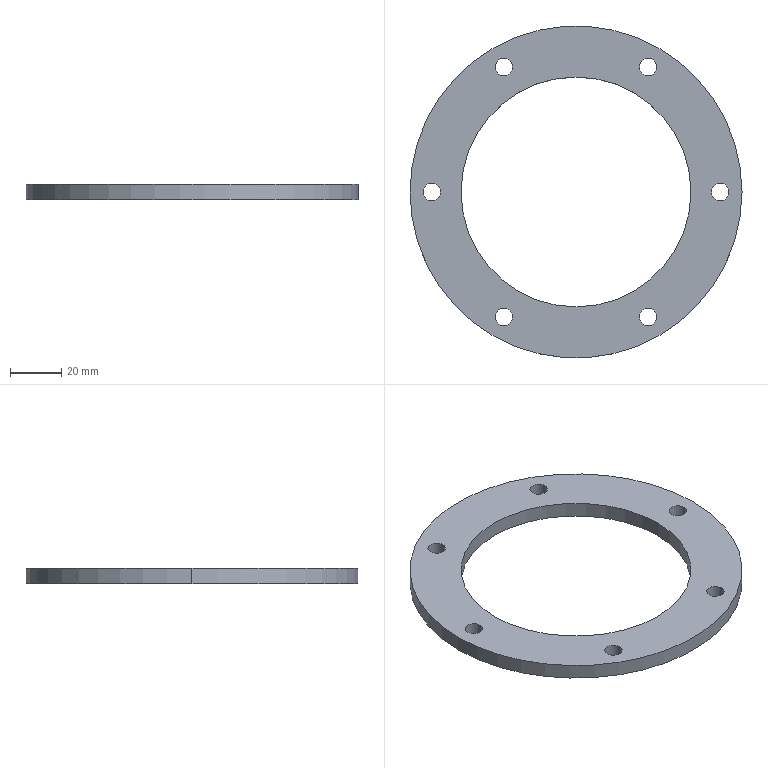Part | SolidWorks | features FlatPattern 1, HoleWzd 1, SMBaseFlange 1, SheetMetal 1 | 1 solid | 18 faces | box 130 x 130 x 6 mm | volume 40162 mm3 | cylinder 16 | plane 2 | commonest cylinder face diameters 6.8 x12 90 x2 130 x2
STEP:
#1=CARTESIAN_POINT('',(-31.65,48.93,-6.));
#2=VERTEX_POINT('',#1);
#3=CARTESIAN_POINT('',(-24.85,48.93,-6.));
#4=VERTEX_POINT('',#3);
#5=CARTESIAN_POINT('',(-28.25,48.93,-6.));
#6=DIRECTION('',(0.,0.,1.));
#7=DIRECTION('',(1.,0.,0.));
#8=AXIS2_PLACEMENT_3D('',#5,#6,#7);
#9=CIRCLE('',#8,3.4);
#10=EDGE_CURVE('',#2,#4,#9,.T.);
#11=ORIENTED_EDGE('',*,*,#10,.F.);
#12=CARTESIAN_POINT('',(-31.65,48.93,0.));
#13=VERTEX_POINT('',#12);
#14=CARTESIAN_POINT('',(-31.65,48.93,0.));
#15=DIRECTION('',(0.,0.,1.));
#16=VECTOR('',#15,1000.);
#17=LINE('',#14,#16);
#18=EDGE_CURVE('',#2,#13,#17,.T.);
#19=ORIENTED_EDGE('',*,*,#18,.T.);
#20=CARTESIAN_POINT('',(-24.85,48.93,0.));
#21=VERTEX_POINT('',#20);
#22=CARTESIAN_POINT('',(-28.25,48.93,0.));
#23=DIRECTION('',(0.,0.,1.));
#24=DIRECTION('',(1.,0.,0.));
#25=AXIS2_PLACEMENT_3D('',#22,#23,#24);
#26=CIRCLE('',#25,3.4);
#27=EDGE_CURVE('',#13,#21,#26,.T.);
#28=ORIENTED_EDGE('',*,*,#27,.T.);
#29=CARTESIAN_POINT('',(-24.85,48.93,0.));
#30=DIRECTION('',(0.,0.,1.));
#31=VECTOR('',#30,1000.);
#32=LINE('',#29,#31);
#33=EDGE_CURVE('',#4,#21,#32,.T.);
#34=ORIENTED_EDGE('',*,*,#33,.F.);
#35=EDGE_LOOP('',(#11,#19,#28,#34));
#36=FACE_OUTER_BOUND('',#35,.T.);
#37=CARTESIAN_POINT('',(-28.25,48.93,0.));
#38=DIRECTION('',(0.,0.,1.));
#39=DIRECTION('',(1.,0.,0.));
#40=AXIS2_PLACEMENT_3D('',#37,#38,#39);
#41=CYLINDRICAL_SURFACE('',#40,3.4);
#42=ADVANCED_FACE('',(#36),#41,.F.);
#43=CARTESIAN_POINT('',(24.85,48.93,-6.));
#44=VERTEX_POINT('',#43);
#45=CARTESIAN_POINT('',(31.65,48.93,-6.));
#46=VERTEX_POINT('',#45);
#47=CARTESIAN_POINT('',(28.25,48.93,-6.));
#48=DIRECTION('',(0.,0.,1.));
#49=DIRECTION('',(1.,0.,0.));
#50=AXIS2_PLACEMENT_3D('',#47,#48,#49);
#51=CIRCLE('',#50,3.4);
#52=EDGE_CURVE('',#44,#46,#51,.T.);
#53=ORIENTED_EDGE('',*,*,#52,.F.);
#54=CARTESIAN_POINT('',(24.85,48.93,0.));
#55=VERTEX_POINT('',#54);
#56=CARTESIAN_POINT('',(24.85,48.93,0.));
#57=DIRECTION('',(0.,0.,1.));
#58=VECTOR('',#57,1000.);
#59=LINE('',#56,#58);
#60=EDGE_CURVE('',#44,#55,#59,.T.);
#61=ORIENTED_EDGE('',*,*,#60,.T.);
#62=CARTESIAN_POINT('',(31.65,48.93,0.));
#63=VERTEX_POINT('',#62);
#64=CARTESIAN_POINT('',(28.25,48.93,0.));
#65=DIRECTION('',(0.,0.,1.));
#66=DIRECTION('',(1.,0.,0.));
#67=AXIS2_PLACEMENT_3D('',#64,#65,#66);
#68=CIRCLE('',#67,3.4);
#69=EDGE_CURVE('',#55,#63,#68,.T.);
#70=ORIENTED_EDGE('',*,*,#69,.T.);
#71=CARTESIAN_POINT('',(31.65,48.93,0.));
#72=DIRECTION('',(0.,0.,1.));
#73=VECTOR('',#72,1000.);
#74=LINE('',#71,#73);
#75=EDGE_CURVE('',#46,#63,#74,.T.);
#76=ORIENTED_EDGE('',*,*,#75,.F.);
#77=EDGE_LOOP('',(#53,#61,#70,#76));
#78=FACE_OUTER_BOUND('',#77,.T.);
#79=CARTESIAN_POINT('',(28.25,48.93,0.));
#80=DIRECTION('',(0.,0.,1.));
#81=DIRECTION('',(1.,0.,0.));
#82=AXIS2_PLACEMENT_3D('',#79,#80,#81);
#83=CYLINDRICAL_SURFACE('',#82,3.4);
#84=ADVANCED_FACE('',(#78),#83,.F.);
#85=CARTESIAN_POINT('',(53.1,0.,-6.));
#86=VERTEX_POINT('',#85);
#87=CARTESIAN_POINT('',(59.9,0.,-6.));
#88=VERTEX_POINT('',#87);
#89=CARTESIAN_POINT('',(56.5,0.,-6.));
#90=DIRECTION('',(0.,0.,1.));
#91=DIRECTION('',(1.,0.,0.));
#92=AXIS2_PLACEMENT_3D('',#89,#90,#91);
#93=CIRCLE('',#92,3.4);
#94=EDGE_CURVE('',#86,#88,#93,.T.);
#95=ORIENTED_EDGE('',*,*,#94,.F.);
#96=CARTESIAN_POINT('',(53.1,0.,0.));
#97=VERTEX_POINT('',#96);
#98=CARTESIAN_POINT('',(53.1,0.,0.));
#99=DIRECTION('',(0.,0.,1.));
#100=VECTOR('',#99,1000.);
#101=LINE('',#98,#100);
#102=EDGE_CURVE('',#86,#97,#101,.T.);
#103=ORIENTED_EDGE('',*,*,#102,.T.);
#104=CARTESIAN_POINT('',(59.9,0.,0.));
#105=VERTEX_POINT('',#104);
#106=CARTESIAN_POINT('',(56.5,0.,0.));
#107=DIRECTION('',(0.,0.,1.));
#108=DIRECTION('',(1.,0.,0.));
#109=AXIS2_PLACEMENT_3D('',#106,#107,#108);
#110=CIRCLE('',#109,3.4);
#111=EDGE_CURVE('',#97,#105,#110,.T.);
#112=ORIENTED_EDGE('',*,*,#111,.T.);
#113=CARTESIAN_POINT('',(59.9,0.,0.));
#114=DIRECTION('',(0.,0.,1.));
#115=VECTOR('',#114,1000.);
#116=LINE('',#113,#115);
#117=EDGE_CURVE('',#88,#105,#116,.T.);
#118=ORIENTED_EDGE('',*,*,#117,.F.);
#119=EDGE_LOOP('',(#95,#103,#112,#118));
#120=FACE_OUTER_BOUND('',#119,.T.);
#121=CARTESIAN_POINT('',(56.5,0.,0.));
#122=DIRECTION('',(0.,0.,1.));
#123=DIRECTION('',(1.,0.,0.));
#124=AXIS2_PLACEMENT_3D('',#121,#122,#123);
#125=CYLINDRICAL_SURFACE('',#124,3.4);
#126=ADVANCED_FACE('',(#120),#125,.F.);
#127=CARTESIAN_POINT('',(-59.9,0.,-6.));
#128=VERTEX_POINT('',#127);
#129=CARTESIAN_POINT('',(-53.1,0.,-6.));
#130=VERTEX_POINT('',#129);
#131=CARTESIAN_POINT('',(-56.5,0.,-6.));
#132=DIRECTION('',(0.,0.,1.));
#133=DIRECTION('',(1.,0.,0.));
#134=AXIS2_PLACEMENT_3D('',#131,#132,#133);
#135=CIRCLE('',#134,3.4);
#136=EDGE_CURVE('',#128,#130,#135,.T.);
#137=ORIENTED_EDGE('',*,*,#136,.F.);
#138=CARTESIAN_POINT('',(-59.9,0.,0.));
#139=VERTEX_POINT('',#138);
#140=CARTESIAN_POINT('',(-59.9,0.,0.));
#141=DIRECTION('',(0.,0.,1.));
#142=VECTOR('',#141,1000.);
#143=LINE('',#140,#142);
#144=EDGE_CURVE('',#128,#139,#143,.T.);
#145=ORIENTED_EDGE('',*,*,#144,.T.);
#146=CARTESIAN_POINT('',(-53.1,0.,0.));
#147=VERTEX_POINT('',#146);
#148=CARTESIAN_POINT('',(-56.5,0.,0.));
#149=DIRECTION('',(0.,0.,1.));
#150=DIRECTION('',(1.,0.,0.));
#151=AXIS2_PLACEMENT_3D('',#148,#149,#150);
#152=CIRCLE('',#151,3.4);
#153=EDGE_CURVE('',#139,#147,#152,.T.);
#154=ORIENTED_EDGE('',*,*,#153,.T.);
#155=CARTESIAN_POINT('',(-53.1,0.,0.));
#156=DIRECTION('',(0.,0.,1.));
#157=VECTOR('',#156,1000.);
#158=LINE('',#155,#157);
#159=EDGE_CURVE('',#130,#147,#158,.T.);
#160=ORIENTED_EDGE('',*,*,#159,.F.);
#161=EDGE_LOOP('',(#137,#145,#154,#160));
#162=FACE_OUTER_BOUND('',#161,.T.);
#163=CARTESIAN_POINT('',(-56.5,0.,0.));
#164=DIRECTION('',(0.,0.,1.));
#165=DIRECTION('',(1.,0.,0.));
#166=AXIS2_PLACEMENT_3D('',#163,#164,#165);
#167=CYLINDRICAL_SURFACE('',#166,3.4);
#168=ADVANCED_FACE('',(#162),#167,.F.);
#169=CARTESIAN_POINT('',(-31.65,-48.93,-6.));
#170=VERTEX_POINT('',#169);
#171=CARTESIAN_POINT('',(-24.85,-48.93,-6.));
#172=VERTEX_POINT('',#171);
#173=CARTESIAN_POINT('',(-28.25,-48.93,-6.));
#174=DIRECTION('',(0.,0.,1.));
#175=DIRECTION('',(1.,0.,0.));
#176=AXIS2_PLACEMENT_3D('',#173,#174,#175);
#177=CIRCLE('',#176,3.4);
#178=EDGE_CURVE('',#170,#172,#177,.T.);
#179=ORIENTED_EDGE('',*,*,#178,.F.);
#180=CARTESIAN_POINT('',(-31.65,-48.93,0.));
#181=VERTEX_POINT('',#180);
#182=CARTESIAN_POINT('',(-31.65,-48.93,0.));
#183=DIRECTION('',(0.,0.,1.));
#184=VECTOR('',#183,1000.);
#185=LINE('',#182,#184);
#186=EDGE_CURVE('',#170,#181,#185,.T.);
#187=ORIENTED_EDGE('',*,*,#186,.T.);
#188=CARTESIAN_POINT('',(-24.85,-48.93,0.));
#189=VERTEX_POINT('',#188);
#190=CARTESIAN_POINT('',(-28.25,-48.93,0.));
#191=DIRECTION('',(0.,0.,1.));
#192=DIRECTION('',(1.,0.,0.));
#193=AXIS2_PLACEMENT_3D('',#190,#191,#192);
#194=CIRCLE('',#193,3.4);
#195=EDGE_CURVE('',#181,#189,#194,.T.);
#196=ORIENTED_EDGE('',*,*,#195,.T.);
#197=CARTESIAN_POINT('',(-24.85,-48.93,0.));
#198=DIRECTION('',(0.,0.,1.));
#199=VECTOR('',#198,1000.);
#200=LINE('',#197,#199);
#201=EDGE_CURVE('',#172,#189,#200,.T.);
#202=ORIENTED_EDGE('',*,*,#201,.F.);
#203=EDGE_LOOP('',(#179,#187,#196,#202));
#204=FACE_OUTER_BOUND('',#203,.T.);
#205=CARTESIAN_POINT('',(-28.25,-48.93,0.));
#206=DIRECTION('',(0.,0.,1.));
#207=DIRECTION('',(1.,0.,0.));
#208=AXIS2_PLACEMENT_3D('',#205,#206,#207);
#209=CYLINDRICAL_SURFACE('',#208,3.4);
#210=ADVANCED_FACE('',(#204),#209,.F.);
#211=CARTESIAN_POINT('',(24.85,-48.93,-6.));
#212=VERTEX_POINT('',#211);
#213=CARTESIAN_POINT('',(31.65,-48.93,-6.));
#214=VERTEX_POINT('',#213);
#215=CARTESIAN_POINT('',(28.25,-48.93,-6.));
#216=DIRECTION('',(0.,0.,1.));
#217=DIRECTION('',(1.,0.,0.));
#218=AXIS2_PLACEMENT_3D('',#215,#216,#217);
#219=CIRCLE('',#218,3.4);
#220=EDGE_CURVE('',#212,#214,#219,.T.);
#221=ORIENTED_EDGE('',*,*,#220,.F.);
#222=CARTESIAN_POINT('',(24.85,-48.93,0.));
#223=VERTEX_POINT('',#222);
#224=CARTESIAN_POINT('',(24.85,-48.93,0.));
#225=DIRECTION('',(0.,0.,1.));
#226=VECTOR('',#225,1000.);
#227=LINE('',#224,#226);
#228=EDGE_CURVE('',#212,#223,#227,.T.);
#229=ORIENTED_EDGE('',*,*,#228,.T.);
#230=CARTESIAN_POINT('',(31.65,-48.93,0.));
#231=VERTEX_POINT('',#230);
#232=CARTESIAN_POINT('',(28.25,-48.93,0.));
#233=DIRECTION('',(0.,0.,1.));
#234=DIRECTION('',(1.,0.,0.));
#235=AXIS2_PLACEMENT_3D('',#232,#233,#234);
#236=CIRCLE('',#235,3.4);
#237=EDGE_CURVE('',#223,#231,#236,.T.);
#238=ORIENTED_EDGE('',*,*,#237,.T.);
#239=CARTESIAN_POINT('',(31.65,-48.93,0.));
#240=DIRECTION('',(0.,0.,1.));
#241=VECTOR('',#240,1000.);
#242=LINE('',#239,#241);
#243=EDGE_CURVE('',#214,#231,#242,.T.);
#244=ORIENTED_EDGE('',*,*,#243,.F.);
#245=EDGE_LOOP('',(#221,#229,#238,#244));
#246=FACE_OUTER_BOUND('',#245,.T.);
#247=CARTESIAN_POINT('',(28.25,-48.93,0.));
#248=DIRECTION('',(0.,0.,1.));
#249=DIRECTION('',(1.,0.,0.));
#250=AXIS2_PLACEMENT_3D('',#247,#248,#249);
#251=CYLINDRICAL_SURFACE('',#250,3.4);
#252=ADVANCED_FACE('',(#246),#251,.F.);
#253=CARTESIAN_POINT('',(-45.,0.,-6.));
#254=VERTEX_POINT('',#253);
#255=CARTESIAN_POINT('',(45.,0.,-6.));
#256=VERTEX_POINT('',#255);
#257=CARTESIAN_POINT('',(0.,0.,-6.));
#258=DIRECTION('',(0.,0.,1.));
#259=DIRECTION('',(1.,0.,0.));
#260=AXIS2_PLACEMENT_3D('',#257,#258,#259);
#261=CIRCLE('',#260,45.);
#262=EDGE_CURVE('',#254,#256,#261,.T.);
#263=ORIENTED_EDGE('',*,*,#262,.F.);
#264=CARTESIAN_POINT('',(-45.,0.,0.));
#265=VERTEX_POINT('',#264);
#266=CARTESIAN_POINT('',(-45.,0.,-6.));
#267=DIRECTION('',(0.,0.,1.));
#268=VECTOR('',#267,1000.);
#269=LINE('',#266,#268);
#270=EDGE_CURVE('',#254,#265,#269,.T.);
#271=ORIENTED_EDGE('',*,*,#270,.T.);
#272=CARTESIAN_POINT('',(45.,0.,0.));
#273=VERTEX_POINT('',#272);
#274=CARTESIAN_POINT('',(0.,0.,0.));
#275=DIRECTION('',(0.,0.,1.));
#276=DIRECTION('',(1.,0.,0.));
#277=AXIS2_PLACEMENT_3D('',#274,#275,#276);
#278=CIRCLE('',#277,45.);
#279=EDGE_CURVE('',#265,#273,#278,.T.);
#280=ORIENTED_EDGE('',*,*,#279,.T.);
#281=CARTESIAN_POINT('',(45.,0.,-6.));
#282=DIRECTION('',(0.,0.,1.));
#283=VECTOR('',#282,1000.);
#284=LINE('',#281,#283);
#285=EDGE_CURVE('',#256,#273,#284,.T.);
#286=ORIENTED_EDGE('',*,*,#285,.F.);
#287=EDGE_LOOP('',(#263,#271,#280,#286));
#288=FACE_OUTER_BOUND('',#287,.T.);
#289=CARTESIAN_POINT('',(0.,0.,-6.));
#290=DIRECTION('',(0.,0.,1.));
#291=DIRECTION('',(1.,0.,0.));
#292=AXIS2_PLACEMENT_3D('',#289,#290,#291);
#293=CYLINDRICAL_SURFACE('',#292,45.);
#294=ADVANCED_FACE('',(#288),#293,.F.);
#295=CARTESIAN_POINT('',(65.,0.,-6.));
#296=VERTEX_POINT('',#295);
#297=CARTESIAN_POINT('',(-65.,0.,-6.));
#298=VERTEX_POINT('',#297);
#299=CARTESIAN_POINT('',(0.,0.,-6.));
#300=DIRECTION('',(0.,0.,1.));
#301=DIRECTION('',(1.,0.,0.));
#302=AXIS2_PLACEMENT_3D('',#299,#300,#301);
#303=CIRCLE('',#302,65.);
#304=EDGE_CURVE('',#296,#298,#303,.T.);
#305=ORIENTED_EDGE('',*,*,#304,.T.);
#306=CARTESIAN_POINT('',(-65.,0.,0.));
#307=VERTEX_POINT('',#306);
#308=CARTESIAN_POINT('',(-65.,0.,-6.));
#309=DIRECTION('',(0.,0.,1.));
#310=VECTOR('',#309,1000.);
#311=LINE('',#308,#310);
#312=EDGE_CURVE('',#298,#307,#311,.T.);
#313=ORIENTED_EDGE('',*,*,#312,.T.);
#314=CARTESIAN_POINT('',(65.,0.,0.));
#315=VERTEX_POINT('',#314);
#316=CARTESIAN_POINT('',(0.,0.,0.));
#317=DIRECTION('',(0.,0.,1.));
#318=DIRECTION('',(1.,0.,0.));
#319=AXIS2_PLACEMENT_3D('',#316,#317,#318);
#320=CIRCLE('',#319,65.);
#321=EDGE_CURVE('',#315,#307,#320,.T.);
#322=ORIENTED_EDGE('',*,*,#321,.F.);
#323=CARTESIAN_POINT('',(65.,0.,-6.));
#324=DIRECTION('',(0.,0.,1.));
#325=VECTOR('',#324,1000.);
#326=LINE('',#323,#325);
#327=EDGE_CURVE('',#296,#315,#326,.T.);
#328=ORIENTED_EDGE('',*,*,#327,.F.);
#329=EDGE_LOOP('',(#305,#313,#322,#328));
#330=FACE_OUTER_BOUND('',#329,.T.);
#331=CARTESIAN_POINT('',(0.,0.,-6.));
#332=DIRECTION('',(0.,0.,1.));
#333=DIRECTION('',(1.,0.,0.));
#334=AXIS2_PLACEMENT_3D('',#331,#332,#333);
#335=CYLINDRICAL_SURFACE('',#334,65.);
#336=ADVANCED_FACE('',(#330),#335,.T.);
#337=ORIENTED_EDGE('',*,*,#312,.F.);
#338=CARTESIAN_POINT('',(0.,0.,-6.));
#339=DIRECTION('',(0.,0.,1.));
#340=DIRECTION('',(1.,0.,0.));
#341=AXIS2_PLACEMENT_3D('',#338,#339,#340);
#342=CIRCLE('',#341,65.);
#343=EDGE_CURVE('',#298,#296,#342,.T.);
#344=ORIENTED_EDGE('',*,*,#343,.T.);
#345=ORIENTED_EDGE('',*,*,#327,.T.);
#346=CARTESIAN_POINT('',(0.,0.,0.));
#347=DIRECTION('',(0.,0.,1.));
#348=DIRECTION('',(1.,0.,0.));
#349=AXIS2_PLACEMENT_3D('',#346,#347,#348);
#350=CIRCLE('',#349,65.);
#351=EDGE_CURVE('',#307,#315,#350,.T.);
#352=ORIENTED_EDGE('',*,*,#351,.F.);
#353=EDGE_LOOP('',(#337,#344,#345,#352));
#354=FACE_OUTER_BOUND('',#353,.T.);
#355=CARTESIAN_POINT('',(0.,0.,-6.));
#356=DIRECTION('',(0.,0.,1.));
#357=DIRECTION('',(1.,0.,0.));
#358=AXIS2_PLACEMENT_3D('',#355,#356,#357);
#359=CYLINDRICAL_SURFACE('',#358,65.);
#360=ADVANCED_FACE('',(#354),#359,.T.);
#361=CARTESIAN_POINT('',(-28.25,48.93,-6.));
#362=DIRECTION('',(0.,0.,1.));
#363=DIRECTION('',(1.,0.,0.));
#364=AXIS2_PLACEMENT_3D('',#361,#362,#363);
#365=CIRCLE('',#364,3.4);
#366=EDGE_CURVE('',#4,#2,#365,.T.);
#367=ORIENTED_EDGE('',*,*,#366,.T.);
#368=ORIENTED_EDGE('',*,*,#10,.T.);
#369=EDGE_LOOP('',(#367,#368));
#370=FACE_BOUND('',#369,.T.);
#371=CARTESIAN_POINT('',(28.25,48.93,-6.));
#372=DIRECTION('',(0.,0.,1.));
#373=DIRECTION('',(1.,0.,0.));
#374=AXIS2_PLACEMENT_3D('',#371,#372,#373);
#375=CIRCLE('',#374,3.4);
#376=EDGE_CURVE('',#46,#44,#375,.T.);
#377=ORIENTED_EDGE('',*,*,#376,.T.);
#378=ORIENTED_EDGE('',*,*,#52,.T.);
#379=EDGE_LOOP('',(#377,#378));
#380=FACE_BOUND('',#379,.T.);
#381=CARTESIAN_POINT('',(56.5,0.,-6.));
#382=DIRECTION('',(0.,0.,1.));
#383=DIRECTION('',(1.,0.,0.));
#384=AXIS2_PLACEMENT_3D('',#381,#382,#383);
#385=CIRCLE('',#384,3.4);
#386=EDGE_CURVE('',#88,#86,#385,.T.);
#387=ORIENTED_EDGE('',*,*,#386,.T.);
#388=ORIENTED_EDGE('',*,*,#94,.T.);
#389=EDGE_LOOP('',(#387,#388));
#390=FACE_BOUND('',#389,.T.);
#391=CARTESIAN_POINT('',(-56.5,0.,-6.));
#392=DIRECTION('',(0.,0.,1.));
#393=DIRECTION('',(1.,0.,0.));
#394=AXIS2_PLACEMENT_3D('',#391,#392,#393);
#395=CIRCLE('',#394,3.4);
#396=EDGE_CURVE('',#130,#128,#395,.T.);
#397=ORIENTED_EDGE('',*,*,#396,.T.);
#398=ORIENTED_EDGE('',*,*,#136,.T.);
#399=EDGE_LOOP('',(#397,#398));
#400=FACE_BOUND('',#399,.T.);
#401=CARTESIAN_POINT('',(-28.25,-48.93,-6.));
#402=DIRECTION('',(0.,0.,1.));
#403=DIRECTION('',(1.,0.,0.));
#404=AXIS2_PLACEMENT_3D('',#401,#402,#403);
#405=CIRCLE('',#404,3.4);
#406=EDGE_CURVE('',#172,#170,#405,.T.);
#407=ORIENTED_EDGE('',*,*,#406,.T.);
#408=ORIENTED_EDGE('',*,*,#178,.T.);
#409=EDGE_LOOP('',(#407,#408));
#410=FACE_BOUND('',#409,.T.);
#411=CARTESIAN_POINT('',(28.25,-48.93,-6.));
#412=DIRECTION('',(0.,0.,1.));
#413=DIRECTION('',(1.,0.,0.));
#414=AXIS2_PLACEMENT_3D('',#411,#412,#413);
#415=CIRCLE('',#414,3.4);
#416=EDGE_CURVE('',#214,#212,#415,.T.);
#417=ORIENTED_EDGE('',*,*,#416,.T.);
#418=ORIENTED_EDGE('',*,*,#220,.T.);
#419=EDGE_LOOP('',(#417,#418));
#420=FACE_BOUND('',#419,.T.);
#421=CARTESIAN_POINT('',(0.,0.,-6.));
#422=DIRECTION('',(0.,0.,1.));
#423=DIRECTION('',(1.,0.,0.));
#424=AXIS2_PLACEMENT_3D('',#421,#422,#423);
#425=CIRCLE('',#424,45.);
#426=EDGE_CURVE('',#256,#254,#425,.T.);
#427=ORIENTED_EDGE('',*,*,#426,.T.);
#428=ORIENTED_EDGE('',*,*,#262,.T.);
#429=EDGE_LOOP('',(#427,#428));
#430=FACE_BOUND('',#429,.T.);
#431=ORIENTED_EDGE('',*,*,#304,.F.);
#432=ORIENTED_EDGE('',*,*,#343,.F.);
#433=EDGE_LOOP('',(#431,#432));
#434=FACE_OUTER_BOUND('',#433,.T.);
#435=CARTESIAN_POINT('',(0.,0.,-6.));
#436=DIRECTION('',(0.,0.,1.));
#437=DIRECTION('',(1.,0.,0.));
#438=AXIS2_PLACEMENT_3D('',#435,#436,#437);
#439=PLANE('',#438);
#440=ADVANCED_FACE('',(#370,#380,#390,#400,#410,#420,#430,#434),#439,.F.);
#441=CARTESIAN_POINT('',(-28.25,48.93,0.));
#442=DIRECTION('',(0.,0.,1.));
#443=DIRECTION('',(1.,0.,0.));
#444=AXIS2_PLACEMENT_3D('',#441,#442,#443);
#445=CIRCLE('',#444,3.4);
#446=EDGE_CURVE('',#21,#13,#445,.T.);
#447=ORIENTED_EDGE('',*,*,#446,.F.);
#448=ORIENTED_EDGE('',*,*,#27,.F.);
#449=EDGE_LOOP('',(#447,#448));
#450=FACE_BOUND('',#449,.T.);
#451=CARTESIAN_POINT('',(28.25,48.93,0.));
#452=DIRECTION('',(0.,0.,1.));
#453=DIRECTION('',(1.,0.,0.));
#454=AXIS2_PLACEMENT_3D('',#451,#452,#453);
#455=CIRCLE('',#454,3.4);
#456=EDGE_CURVE('',#63,#55,#455,.T.);
#457=ORIENTED_EDGE('',*,*,#456,.F.);
#458=ORIENTED_EDGE('',*,*,#69,.F.);
#459=EDGE_LOOP('',(#457,#458));
#460=FACE_BOUND('',#459,.T.);
#461=CARTESIAN_POINT('',(56.5,0.,0.));
#462=DIRECTION('',(0.,0.,1.));
#463=DIRECTION('',(1.,0.,0.));
#464=AXIS2_PLACEMENT_3D('',#461,#462,#463);
#465=CIRCLE('',#464,3.4);
#466=EDGE_CURVE('',#105,#97,#465,.T.);
#467=ORIENTED_EDGE('',*,*,#466,.F.);
#468=ORIENTED_EDGE('',*,*,#111,.F.);
#469=EDGE_LOOP('',(#467,#468));
#470=FACE_BOUND('',#469,.T.);
#471=CARTESIAN_POINT('',(-56.5,0.,0.));
#472=DIRECTION('',(0.,0.,1.));
#473=DIRECTION('',(1.,0.,0.));
#474=AXIS2_PLACEMENT_3D('',#471,#472,#473);
#475=CIRCLE('',#474,3.4);
#476=EDGE_CURVE('',#147,#139,#475,.T.);
#477=ORIENTED_EDGE('',*,*,#476,.F.);
#478=ORIENTED_EDGE('',*,*,#153,.F.);
#479=EDGE_LOOP('',(#477,#478));
#480=FACE_BOUND('',#479,.T.);
#481=CARTESIAN_POINT('',(-28.25,-48.93,0.));
#482=DIRECTION('',(0.,0.,1.));
#483=DIRECTION('',(1.,0.,0.));
#484=AXIS2_PLACEMENT_3D('',#481,#482,#483);
#485=CIRCLE('',#484,3.4);
#486=EDGE_CURVE('',#189,#181,#485,.T.);
#487=ORIENTED_EDGE('',*,*,#486,.F.);
#488=ORIENTED_EDGE('',*,*,#195,.F.);
#489=EDGE_LOOP('',(#487,#488));
#490=FACE_BOUND('',#489,.T.);
#491=CARTESIAN_POINT('',(28.25,-48.93,0.));
#492=DIRECTION('',(0.,0.,1.));
#493=DIRECTION('',(1.,0.,0.));
#494=AXIS2_PLACEMENT_3D('',#491,#492,#493);
#495=CIRCLE('',#494,3.4);
#496=EDGE_CURVE('',#231,#223,#495,.T.);
#497=ORIENTED_EDGE('',*,*,#496,.F.);
#498=ORIENTED_EDGE('',*,*,#237,.F.);
#499=EDGE_LOOP('',(#497,#498));
#500=FACE_BOUND('',#499,.T.);
#501=CARTESIAN_POINT('',(0.,0.,0.));
#502=DIRECTION('',(0.,0.,1.));
#503=DIRECTION('',(1.,0.,0.));
#504=AXIS2_PLACEMENT_3D('',#501,#502,#503);
#505=CIRCLE('',#504,45.);
#506=EDGE_CURVE('',#273,#265,#505,.T.);
#507=ORIENTED_EDGE('',*,*,#506,.F.);
#508=ORIENTED_EDGE('',*,*,#279,.F.);
#509=EDGE_LOOP('',(#507,#508));
#510=FACE_BOUND('',#509,.T.);
#511=ORIENTED_EDGE('',*,*,#321,.T.);
#512=ORIENTED_EDGE('',*,*,#351,.T.);
#513=EDGE_LOOP('',(#511,#512));
#514=FACE_OUTER_BOUND('',#513,.T.);
#515=CARTESIAN_POINT('',(0.,0.,0.));
#516=DIRECTION('',(0.,0.,1.));
#517=DIRECTION('',(1.,0.,0.));
#518=AXIS2_PLACEMENT_3D('',#515,#516,#517);
#519=PLANE('',#518);
#520=ADVANCED_FACE('',(#450,#460,#470,#480,#490,#500,#510,#514),#519,.T.);
#521=ORIENTED_EDGE('',*,*,#270,.F.);
#522=ORIENTED_EDGE('',*,*,#426,.F.);
#523=ORIENTED_EDGE('',*,*,#285,.T.);
#524=ORIENTED_EDGE('',*,*,#506,.T.);
#525=EDGE_LOOP('',(#521,#522,#523,#524));
#526=FACE_OUTER_BOUND('',#525,.T.);
#527=CARTESIAN_POINT('',(0.,0.,-6.));
#528=DIRECTION('',(0.,0.,1.));
#529=DIRECTION('',(1.,0.,0.));
#530=AXIS2_PLACEMENT_3D('',#527,#528,#529);
#531=CYLINDRICAL_SURFACE('',#530,45.);
#532=ADVANCED_FACE('',(#526),#531,.F.);
#533=ORIENTED_EDGE('',*,*,#228,.F.);
#534=ORIENTED_EDGE('',*,*,#416,.F.);
#535=ORIENTED_EDGE('',*,*,#243,.T.);
#536=ORIENTED_EDGE('',*,*,#496,.T.);
#537=EDGE_LOOP('',(#533,#534,#535,#536));
#538=FACE_OUTER_BOUND('',#537,.T.);
#539=CARTESIAN_POINT('',(28.25,-48.93,0.));
#540=DIRECTION('',(0.,0.,1.));
#541=DIRECTION('',(1.,0.,0.));
#542=AXIS2_PLACEMENT_3D('',#539,#540,#541);
#543=CYLINDRICAL_SURFACE('',#542,3.4);
#544=ADVANCED_FACE('',(#538),#543,.F.);
#545=ORIENTED_EDGE('',*,*,#186,.F.);
#546=ORIENTED_EDGE('',*,*,#406,.F.);
#547=ORIENTED_EDGE('',*,*,#201,.T.);
#548=ORIENTED_EDGE('',*,*,#486,.T.);
#549=EDGE_LOOP('',(#545,#546,#547,#548));
#550=FACE_OUTER_BOUND('',#549,.T.);
#551=CARTESIAN_POINT('',(-28.25,-48.93,0.));
#552=DIRECTION('',(0.,0.,1.));
#553=DIRECTION('',(1.,0.,0.));
#554=AXIS2_PLACEMENT_3D('',#551,#552,#553);
#555=CYLINDRICAL_SURFACE('',#554,3.4);
#556=ADVANCED_FACE('',(#550),#555,.F.);
#557=ORIENTED_EDGE('',*,*,#144,.F.);
#558=ORIENTED_EDGE('',*,*,#396,.F.);
#559=ORIENTED_EDGE('',*,*,#159,.T.);
#560=ORIENTED_EDGE('',*,*,#476,.T.);
#561=EDGE_LOOP('',(#557,#558,#559,#560));
#562=FACE_OUTER_BOUND('',#561,.T.);
#563=CARTESIAN_POINT('',(-56.5,0.,0.));
#564=DIRECTION('',(0.,0.,1.));
#565=DIRECTION('',(1.,0.,0.));
#566=AXIS2_PLACEMENT_3D('',#563,#564,#565);
#567=CYLINDRICAL_SURFACE('',#566,3.4);
#568=ADVANCED_FACE('',(#562),#567,.F.);
#569=ORIENTED_EDGE('',*,*,#102,.F.);
#570=ORIENTED_EDGE('',*,*,#386,.F.);
#571=ORIENTED_EDGE('',*,*,#117,.T.);
#572=ORIENTED_EDGE('',*,*,#466,.T.);
#573=EDGE_LOOP('',(#569,#570,#571,#572));
#574=FACE_OUTER_BOUND('',#573,.T.);
#575=CARTESIAN_POINT('',(56.5,0.,0.));
#576=DIRECTION('',(0.,0.,1.));
#577=DIRECTION('',(1.,0.,0.));
#578=AXIS2_PLACEMENT_3D('',#575,#576,#577);
#579=CYLINDRICAL_SURFACE('',#578,3.4);
#580=ADVANCED_FACE('',(#574),#579,.F.);
#581=ORIENTED_EDGE('',*,*,#60,.F.);
#582=ORIENTED_EDGE('',*,*,#376,.F.);
#583=ORIENTED_EDGE('',*,*,#75,.T.);
#584=ORIENTED_EDGE('',*,*,#456,.T.);
#585=EDGE_LOOP('',(#581,#582,#583,#584));
#586=FACE_OUTER_BOUND('',#585,.T.);
#587=CARTESIAN_POINT('',(28.25,48.93,0.));
#588=DIRECTION('',(0.,0.,1.));
#589=DIRECTION('',(1.,0.,0.));
#590=AXIS2_PLACEMENT_3D('',#587,#588,#589);
#591=CYLINDRICAL_SURFACE('',#590,3.4);
#592=ADVANCED_FACE('',(#586),#591,.F.);
#593=ORIENTED_EDGE('',*,*,#18,.F.);
#594=ORIENTED_EDGE('',*,*,#366,.F.);
#595=ORIENTED_EDGE('',*,*,#33,.T.);
#596=ORIENTED_EDGE('',*,*,#446,.T.);
#597=EDGE_LOOP('',(#593,#594,#595,#596));
#598=FACE_OUTER_BOUND('',#597,.T.);
#599=CARTESIAN_POINT('',(-28.25,48.93,0.));
#600=DIRECTION('',(0.,0.,1.));
#601=DIRECTION('',(1.,0.,0.));
#602=AXIS2_PLACEMENT_3D('',#599,#600,#601);
#603=CYLINDRICAL_SURFACE('',#602,3.4);
#604=ADVANCED_FACE('',(#598),#603,.F.);
#605=CLOSED_SHELL('',(#42,#84,#126,#168,#210,#252,#294,#336,#360,#440,#520,#532,#544,#556,#568,#580,#592,#604));
#606=MANIFOLD_SOLID_BREP('',#605);
#607=CARTESIAN_POINT('',(0.,0.,0.));
#608=DIRECTION('',(0.,0.,1.));
#609=DIRECTION('',(1.,0.,0.));
#610=AXIS2_PLACEMENT_3D('',#607,#608,#609);
#611=(LENGTH_UNIT()NAMED_UNIT(*)SI_UNIT(.MILLI.,.METRE.));
#612=UNCERTAINTY_MEASURE_WITH_UNIT(LENGTH_MEASURE(0.00001),#611,'','');
#613=(NAMED_UNIT(*)PLANE_ANGLE_UNIT()SI_UNIT($,.RADIAN.));
#614=(NAMED_UNIT(*)SI_UNIT($,.STERADIAN.)SOLID_ANGLE_UNIT());
#615=(GEOMETRIC_REPRESENTATION_CONTEXT(3)GLOBAL_UNCERTAINTY_ASSIGNED_CONTEXT((#612))GLOBAL_UNIT_ASSIGNED_CONTEXT((#611,#613,#614))REPRESENTATION_CONTEXT('',''));
#616=ADVANCED_BREP_SHAPE_REPRESENTATION('',(#606,#610),#615);